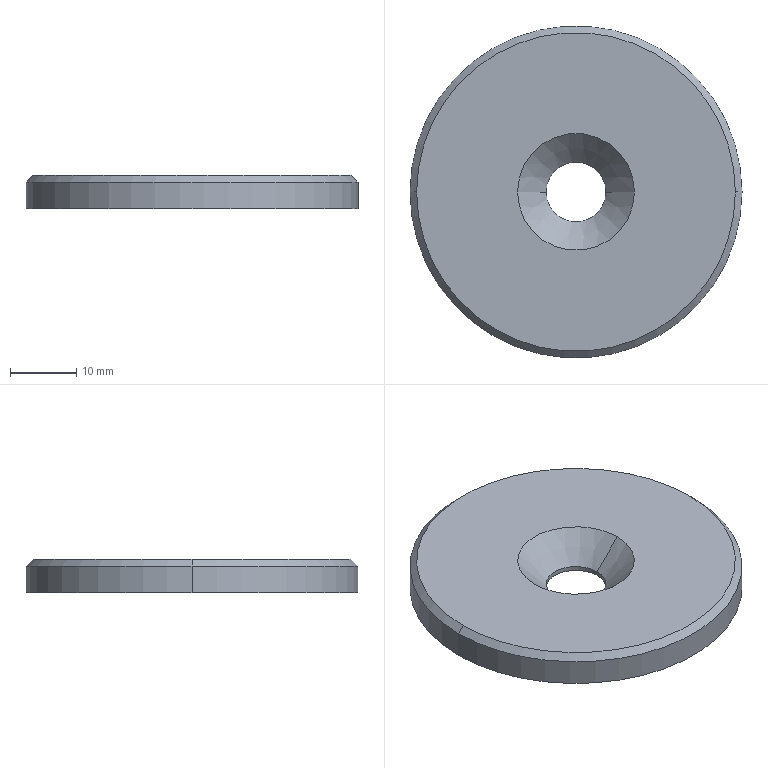Part | SolidWorks | features Chamfer 1, Extrusion 1, HoleWzd 1 | 1 solid | 10 faces | box 50 x 50 x 5 mm | volume 9077 mm3 | cone 4 | cylinder 4 | plane 2 | commonest cylinder face diameters 9 x2 50 x2
STEP:
#1=CARTESIAN_POINT('',(24.,0.,5.));
#2=VERTEX_POINT('',#1);
#3=CARTESIAN_POINT('',(-24.,0.,5.));
#4=VERTEX_POINT('',#3);
#5=CARTESIAN_POINT('',(0.,0.,5.));
#6=DIRECTION('',(0.,0.,1.));
#7=DIRECTION('',(1.,0.,0.));
#8=AXIS2_PLACEMENT_3D('',#5,#6,#7);
#9=CIRCLE('',#8,24.);
#10=EDGE_CURVE('',#2,#4,#9,.T.);
#11=ORIENTED_EDGE('',*,*,#10,.F.);
#12=CARTESIAN_POINT('',(25.,0.,4.));
#13=VERTEX_POINT('',#12);
#14=CARTESIAN_POINT('',(24.,0.,5.));
#15=DIRECTION('',(0.7071,0.,-0.7071));
#16=VECTOR('',#15,1000.);
#17=LINE('',#14,#16);
#18=EDGE_CURVE('',#2,#13,#17,.T.);
#19=ORIENTED_EDGE('',*,*,#18,.T.);
#20=CARTESIAN_POINT('',(-25.,0.,4.));
#21=VERTEX_POINT('',#20);
#22=CARTESIAN_POINT('',(0.,0.,4.));
#23=DIRECTION('',(0.,0.,-1.));
#24=DIRECTION('',(1.,0.,0.));
#25=AXIS2_PLACEMENT_3D('',#22,#23,#24);
#26=CIRCLE('',#25,25.);
#27=EDGE_CURVE('',#21,#13,#26,.T.);
#28=ORIENTED_EDGE('',*,*,#27,.F.);
#29=CARTESIAN_POINT('',(-24.,0.,5.));
#30=DIRECTION('',(-0.7071,0.,-0.7071));
#31=VECTOR('',#30,1000.);
#32=LINE('',#29,#31);
#33=EDGE_CURVE('',#4,#21,#32,.T.);
#34=ORIENTED_EDGE('',*,*,#33,.F.);
#35=EDGE_LOOP('',(#11,#19,#28,#34));
#36=FACE_OUTER_BOUND('',#35,.T.);
#37=CARTESIAN_POINT('',(0.,0.,5.));
#38=DIRECTION('',(0.,0.,-1.));
#39=DIRECTION('',(-1.,0.,0.));
#40=AXIS2_PLACEMENT_3D('',#37,#38,#39);
#41=CONICAL_SURFACE('',#40,24.,0.7854);
#42=ADVANCED_FACE('',(#36),#41,.T.);
#43=CARTESIAN_POINT('',(-4.5,0.,0.7));
#44=VERTEX_POINT('',#43);
#45=CARTESIAN_POINT('',(4.5,0.,0.7));
#46=VERTEX_POINT('',#45);
#47=CARTESIAN_POINT('',(0.,0.,0.7));
#48=DIRECTION('',(0.,0.,1.));
#49=DIRECTION('',(1.,0.,0.));
#50=AXIS2_PLACEMENT_3D('',#47,#48,#49);
#51=CIRCLE('',#50,4.5);
#52=EDGE_CURVE('',#44,#46,#51,.T.);
#53=ORIENTED_EDGE('',*,*,#52,.F.);
#54=CARTESIAN_POINT('',(-8.8,0.,5.));
#55=VERTEX_POINT('',#54);
#56=CARTESIAN_POINT('',(-8.8,0.,5.));
#57=DIRECTION('',(-0.7071,0.,0.7071));
#58=VECTOR('',#57,1000.);
#59=LINE('',#56,#58);
#60=EDGE_CURVE('',#44,#55,#59,.T.);
#61=ORIENTED_EDGE('',*,*,#60,.T.);
#62=CARTESIAN_POINT('',(8.8,0.,5.));
#63=VERTEX_POINT('',#62);
#64=CARTESIAN_POINT('',(0.,0.,5.));
#65=DIRECTION('',(0.,0.,1.));
#66=DIRECTION('',(1.,0.,0.));
#67=AXIS2_PLACEMENT_3D('',#64,#65,#66);
#68=CIRCLE('',#67,8.8);
#69=EDGE_CURVE('',#55,#63,#68,.T.);
#70=ORIENTED_EDGE('',*,*,#69,.T.);
#71=CARTESIAN_POINT('',(8.8,0.,5.));
#72=DIRECTION('',(0.7071,0.,0.7071));
#73=VECTOR('',#72,1000.);
#74=LINE('',#71,#73);
#75=EDGE_CURVE('',#46,#63,#74,.T.);
#76=ORIENTED_EDGE('',*,*,#75,.F.);
#77=EDGE_LOOP('',(#53,#61,#70,#76));
#78=FACE_OUTER_BOUND('',#77,.T.);
#79=CARTESIAN_POINT('',(0.,0.,5.));
#80=DIRECTION('',(0.,0.,1.));
#81=DIRECTION('',(1.,0.,0.));
#82=AXIS2_PLACEMENT_3D('',#79,#80,#81);
#83=CONICAL_SURFACE('',#82,8.8,0.7854);
#84=ADVANCED_FACE('',(#78),#83,.F.);
#85=CARTESIAN_POINT('',(-4.5,0.,0.));
#86=VERTEX_POINT('',#85);
#87=CARTESIAN_POINT('',(4.5,0.,0.));
#88=VERTEX_POINT('',#87);
#89=CARTESIAN_POINT('',(0.,0.,0.));
#90=DIRECTION('',(0.,0.,1.));
#91=DIRECTION('',(1.,0.,0.));
#92=AXIS2_PLACEMENT_3D('',#89,#90,#91);
#93=CIRCLE('',#92,4.5);
#94=EDGE_CURVE('',#86,#88,#93,.T.);
#95=ORIENTED_EDGE('',*,*,#94,.F.);
#96=CARTESIAN_POINT('',(-4.5,0.,5.));
#97=DIRECTION('',(0.,0.,1.));
#98=VECTOR('',#97,1000.);
#99=LINE('',#96,#98);
#100=EDGE_CURVE('',#86,#44,#99,.T.);
#101=ORIENTED_EDGE('',*,*,#100,.T.);
#102=ORIENTED_EDGE('',*,*,#52,.T.);
#103=CARTESIAN_POINT('',(4.5,0.,5.));
#104=DIRECTION('',(0.,0.,1.));
#105=VECTOR('',#104,1000.);
#106=LINE('',#103,#105);
#107=EDGE_CURVE('',#88,#46,#106,.T.);
#108=ORIENTED_EDGE('',*,*,#107,.F.);
#109=EDGE_LOOP('',(#95,#101,#102,#108));
#110=FACE_OUTER_BOUND('',#109,.T.);
#111=CARTESIAN_POINT('',(0.,0.,5.));
#112=DIRECTION('',(0.,0.,1.));
#113=DIRECTION('',(1.,0.,0.));
#114=AXIS2_PLACEMENT_3D('',#111,#112,#113);
#115=CYLINDRICAL_SURFACE('',#114,4.5);
#116=ADVANCED_FACE('',(#110),#115,.F.);
#117=ORIENTED_EDGE('',*,*,#27,.T.);
#118=CARTESIAN_POINT('',(25.,0.,0.));
#119=VERTEX_POINT('',#118);
#120=CARTESIAN_POINT('',(25.,0.,5.));
#121=DIRECTION('',(0.,0.,-1.));
#122=VECTOR('',#121,1000.);
#123=LINE('',#120,#122);
#124=EDGE_CURVE('',#13,#119,#123,.T.);
#125=ORIENTED_EDGE('',*,*,#124,.T.);
#126=CARTESIAN_POINT('',(-25.,0.,0.));
#127=VERTEX_POINT('',#126);
#128=CARTESIAN_POINT('',(0.,0.,0.));
#129=DIRECTION('',(0.,0.,1.));
#130=DIRECTION('',(1.,0.,0.));
#131=AXIS2_PLACEMENT_3D('',#128,#129,#130);
#132=CIRCLE('',#131,25.);
#133=EDGE_CURVE('',#119,#127,#132,.T.);
#134=ORIENTED_EDGE('',*,*,#133,.T.);
#135=CARTESIAN_POINT('',(-25.,0.,5.));
#136=DIRECTION('',(0.,0.,-1.));
#137=VECTOR('',#136,1000.);
#138=LINE('',#135,#137);
#139=EDGE_CURVE('',#21,#127,#138,.T.);
#140=ORIENTED_EDGE('',*,*,#139,.F.);
#141=EDGE_LOOP('',(#117,#125,#134,#140));
#142=FACE_OUTER_BOUND('',#141,.T.);
#143=CARTESIAN_POINT('',(0.,0.,5.));
#144=DIRECTION('',(0.,0.,-1.));
#145=DIRECTION('',(-1.,0.,0.));
#146=AXIS2_PLACEMENT_3D('',#143,#144,#145);
#147=CYLINDRICAL_SURFACE('',#146,25.);
#148=ADVANCED_FACE('',(#142),#147,.T.);
#149=ORIENTED_EDGE('',*,*,#124,.F.);
#150=CARTESIAN_POINT('',(0.,0.,4.));
#151=DIRECTION('',(0.,0.,-1.));
#152=DIRECTION('',(1.,0.,0.));
#153=AXIS2_PLACEMENT_3D('',#150,#151,#152);
#154=CIRCLE('',#153,25.);
#155=EDGE_CURVE('',#13,#21,#154,.T.);
#156=ORIENTED_EDGE('',*,*,#155,.T.);
#157=ORIENTED_EDGE('',*,*,#139,.T.);
#158=CARTESIAN_POINT('',(0.,0.,0.));
#159=DIRECTION('',(0.,0.,1.));
#160=DIRECTION('',(1.,0.,0.));
#161=AXIS2_PLACEMENT_3D('',#158,#159,#160);
#162=CIRCLE('',#161,25.);
#163=EDGE_CURVE('',#127,#119,#162,.T.);
#164=ORIENTED_EDGE('',*,*,#163,.T.);
#165=EDGE_LOOP('',(#149,#156,#157,#164));
#166=FACE_OUTER_BOUND('',#165,.T.);
#167=CARTESIAN_POINT('',(0.,0.,5.));
#168=DIRECTION('',(0.,0.,-1.));
#169=DIRECTION('',(-1.,0.,0.));
#170=AXIS2_PLACEMENT_3D('',#167,#168,#169);
#171=CYLINDRICAL_SURFACE('',#170,25.);
#172=ADVANCED_FACE('',(#166),#171,.T.);
#173=CARTESIAN_POINT('',(0.,0.,5.));
#174=DIRECTION('',(0.,0.,1.));
#175=DIRECTION('',(1.,0.,0.));
#176=AXIS2_PLACEMENT_3D('',#173,#174,#175);
#177=CIRCLE('',#176,24.);
#178=EDGE_CURVE('',#4,#2,#177,.T.);
#179=ORIENTED_EDGE('',*,*,#178,.T.);
#180=ORIENTED_EDGE('',*,*,#10,.T.);
#181=EDGE_LOOP('',(#179,#180));
#182=FACE_OUTER_BOUND('',#181,.T.);
#183=CARTESIAN_POINT('',(0.,0.,5.));
#184=DIRECTION('',(0.,0.,1.));
#185=DIRECTION('',(1.,0.,0.));
#186=AXIS2_PLACEMENT_3D('',#183,#184,#185);
#187=CIRCLE('',#186,8.8);
#188=EDGE_CURVE('',#63,#55,#187,.T.);
#189=ORIENTED_EDGE('',*,*,#188,.F.);
#190=ORIENTED_EDGE('',*,*,#69,.F.);
#191=EDGE_LOOP('',(#189,#190));
#192=FACE_BOUND('',#191,.T.);
#193=CARTESIAN_POINT('',(0.,0.,5.));
#194=DIRECTION('',(0.,0.,1.));
#195=DIRECTION('',(1.,0.,0.));
#196=AXIS2_PLACEMENT_3D('',#193,#194,#195);
#197=PLANE('',#196);
#198=ADVANCED_FACE('',(#182,#192),#197,.T.);
#199=CARTESIAN_POINT('',(0.,0.,0.));
#200=DIRECTION('',(0.,0.,1.));
#201=DIRECTION('',(1.,0.,0.));
#202=AXIS2_PLACEMENT_3D('',#199,#200,#201);
#203=CIRCLE('',#202,4.5);
#204=EDGE_CURVE('',#88,#86,#203,.T.);
#205=ORIENTED_EDGE('',*,*,#204,.T.);
#206=ORIENTED_EDGE('',*,*,#94,.T.);
#207=EDGE_LOOP('',(#205,#206));
#208=FACE_BOUND('',#207,.T.);
#209=ORIENTED_EDGE('',*,*,#163,.F.);
#210=ORIENTED_EDGE('',*,*,#133,.F.);
#211=EDGE_LOOP('',(#209,#210));
#212=FACE_OUTER_BOUND('',#211,.T.);
#213=CARTESIAN_POINT('',(0.,0.,0.));
#214=DIRECTION('',(0.,0.,1.));
#215=DIRECTION('',(1.,0.,0.));
#216=AXIS2_PLACEMENT_3D('',#213,#214,#215);
#217=PLANE('',#216);
#218=ADVANCED_FACE('',(#208,#212),#217,.F.);
#219=ORIENTED_EDGE('',*,*,#100,.F.);
#220=ORIENTED_EDGE('',*,*,#204,.F.);
#221=ORIENTED_EDGE('',*,*,#107,.T.);
#222=CARTESIAN_POINT('',(0.,0.,0.7));
#223=DIRECTION('',(0.,0.,1.));
#224=DIRECTION('',(1.,0.,0.));
#225=AXIS2_PLACEMENT_3D('',#222,#223,#224);
#226=CIRCLE('',#225,4.5);
#227=EDGE_CURVE('',#46,#44,#226,.T.);
#228=ORIENTED_EDGE('',*,*,#227,.T.);
#229=EDGE_LOOP('',(#219,#220,#221,#228));
#230=FACE_OUTER_BOUND('',#229,.T.);
#231=CARTESIAN_POINT('',(0.,0.,5.));
#232=DIRECTION('',(0.,0.,1.));
#233=DIRECTION('',(1.,0.,0.));
#234=AXIS2_PLACEMENT_3D('',#231,#232,#233);
#235=CYLINDRICAL_SURFACE('',#234,4.5);
#236=ADVANCED_FACE('',(#230),#235,.F.);
#237=ORIENTED_EDGE('',*,*,#60,.F.);
#238=ORIENTED_EDGE('',*,*,#227,.F.);
#239=ORIENTED_EDGE('',*,*,#75,.T.);
#240=ORIENTED_EDGE('',*,*,#188,.T.);
#241=EDGE_LOOP('',(#237,#238,#239,#240));
#242=FACE_OUTER_BOUND('',#241,.T.);
#243=CARTESIAN_POINT('',(0.,0.,5.));
#244=DIRECTION('',(0.,0.,1.));
#245=DIRECTION('',(1.,0.,0.));
#246=AXIS2_PLACEMENT_3D('',#243,#244,#245);
#247=CONICAL_SURFACE('',#246,8.8,0.7854);
#248=ADVANCED_FACE('',(#242),#247,.F.);
#249=ORIENTED_EDGE('',*,*,#18,.F.);
#250=ORIENTED_EDGE('',*,*,#178,.F.);
#251=ORIENTED_EDGE('',*,*,#33,.T.);
#252=ORIENTED_EDGE('',*,*,#155,.F.);
#253=EDGE_LOOP('',(#249,#250,#251,#252));
#254=FACE_OUTER_BOUND('',#253,.T.);
#255=CARTESIAN_POINT('',(0.,0.,5.));
#256=DIRECTION('',(0.,0.,-1.));
#257=DIRECTION('',(-1.,0.,0.));
#258=AXIS2_PLACEMENT_3D('',#255,#256,#257);
#259=CONICAL_SURFACE('',#258,24.,0.7854);
#260=ADVANCED_FACE('',(#254),#259,.T.);
#261=CLOSED_SHELL('',(#42,#84,#116,#148,#172,#198,#218,#236,#248,#260));
#262=MANIFOLD_SOLID_BREP('',#261);
#263=CARTESIAN_POINT('',(0.,0.,0.));
#264=DIRECTION('',(0.,0.,1.));
#265=DIRECTION('',(1.,0.,0.));
#266=AXIS2_PLACEMENT_3D('',#263,#264,#265);
#267=(LENGTH_UNIT()NAMED_UNIT(*)SI_UNIT(.MILLI.,.METRE.));
#268=UNCERTAINTY_MEASURE_WITH_UNIT(LENGTH_MEASURE(0.00001),#267,'','');
#269=(NAMED_UNIT(*)PLANE_ANGLE_UNIT()SI_UNIT($,.RADIAN.));
#270=(NAMED_UNIT(*)SI_UNIT($,.STERADIAN.)SOLID_ANGLE_UNIT());
#271=(GEOMETRIC_REPRESENTATION_CONTEXT(3)GLOBAL_UNCERTAINTY_ASSIGNED_CONTEXT((#268))GLOBAL_UNIT_ASSIGNED_CONTEXT((#267,#269,#270))REPRESENTATION_CONTEXT('',''));
#272=ADVANCED_BREP_SHAPE_REPRESENTATION('',(#262,#266),#271);